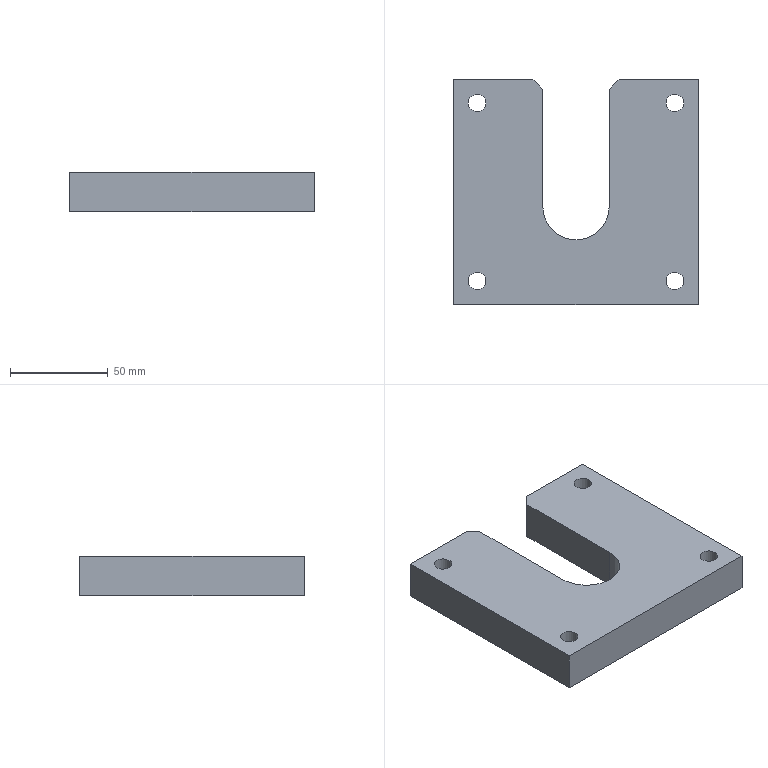Part | NX | features solid 2 | 1 solid | 24 faces | box 125 x 115 x 20 mm | volume 223341 mm3 | plane 15 | cylinder 9 | commonest cylinder face diameters 9.007 x4 14.508 x4 34 x1
STEP:
#1=CARTESIAN_POINT('',(302.977,477.095,246.13));
#2=VERTEX_POINT('',#1);
#3=CARTESIAN_POINT('',(302.977,477.095,226.13));
#4=VERTEX_POINT('',#3);
#5=CARTESIAN_POINT('',(302.977,477.095,221.13));
#6=DIRECTION('',(0.,0.,-1.));
#7=VECTOR('',#6,1000.);
#8=LINE('',#5,#7);
#9=EDGE_CURVE('',#2,#4,#8,.T.);
#10=ORIENTED_EDGE('',*,*,#9,.T.);
#11=CARTESIAN_POINT('',(262.477,477.095,226.13));
#12=VERTEX_POINT('',#11);
#13=CARTESIAN_POINT('',(324.977,477.095,226.13));
#14=DIRECTION('',(1.,0.,0.));
#15=VECTOR('',#14,1000.);
#16=LINE('',#13,#15);
#17=EDGE_CURVE('',#12,#4,#16,.T.);
#18=ORIENTED_EDGE('',*,*,#17,.F.);
#19=CARTESIAN_POINT('',(262.477,477.095,246.13));
#20=VERTEX_POINT('',#19);
#21=CARTESIAN_POINT('',(262.477,477.095,221.13));
#22=DIRECTION('',(0.,0.,1.));
#23=VECTOR('',#22,1000.);
#24=LINE('',#21,#23);
#25=EDGE_CURVE('',#20,#12,#24,.F.);
#26=ORIENTED_EDGE('',*,*,#25,.F.);
#27=CARTESIAN_POINT('',(324.977,477.095,246.13));
#28=DIRECTION('',(1.,0.,0.));
#29=VECTOR('',#28,1000.);
#30=LINE('',#27,#29);
#31=EDGE_CURVE('',#2,#20,#30,.F.);
#32=ORIENTED_EDGE('',*,*,#31,.F.);
#33=EDGE_LOOP('',(#10,#18,#26,#32));
#34=FACE_BOUND('',#33,.T.);
#35=CARTESIAN_POINT('',(324.977,477.095,221.13));
#36=DIRECTION('',(0.,1.,0.));
#37=DIRECTION('',(0.,0.,1.));
#38=AXIS2_PLACEMENT_3D('',#35,#36,#37);
#39=PLANE('',#38);
#40=ADVANCED_FACE('',(#34),#39,.T.);
#41=CARTESIAN_POINT('',(307.977,472.095,226.13));
#42=VERTEX_POINT('',#41);
#43=CARTESIAN_POINT('',(334.227,445.845,226.13));
#44=DIRECTION('',(0.7071,-0.7071,0.));
#45=VECTOR('',#44,1000.);
#46=LINE('',#43,#45);
#47=EDGE_CURVE('',#42,#4,#46,.F.);
#48=ORIENTED_EDGE('',*,*,#47,.F.);
#49=CARTESIAN_POINT('',(307.977,412.095,226.13));
#50=VERTEX_POINT('',#49);
#51=CARTESIAN_POINT('',(307.977,434.595,226.13));
#52=DIRECTION('',(0.,-1.,0.));
#53=VECTOR('',#52,1000.);
#54=LINE('',#51,#53);
#55=EDGE_CURVE('',#42,#50,#54,.T.);
#56=ORIENTED_EDGE('',*,*,#55,.T.);
#57=CARTESIAN_POINT('',(341.977,412.095,226.13));
#58=VERTEX_POINT('',#57);
#59=CARTESIAN_POINT('',(324.977,412.095,226.13));
#60=DIRECTION('',(0.,0.,-1.));
#61=DIRECTION('',(-1.,0.,0.));
#62=AXIS2_PLACEMENT_3D('',#59,#60,#61);
#63=CIRCLE('',#62,17.);
#64=EDGE_CURVE('',#58,#50,#63,.T.);
#65=ORIENTED_EDGE('',*,*,#64,.F.);
#66=CARTESIAN_POINT('',(341.977,472.095,226.13));
#67=VERTEX_POINT('',#66);
#68=CARTESIAN_POINT('',(341.977,434.595,226.13));
#69=DIRECTION('',(0.,1.,0.));
#70=VECTOR('',#69,1000.);
#71=LINE('',#68,#70);
#72=EDGE_CURVE('',#67,#58,#71,.F.);
#73=ORIENTED_EDGE('',*,*,#72,.F.);
#74=CARTESIAN_POINT('',(346.977,477.095,226.13));
#75=VERTEX_POINT('',#74);
#76=CARTESIAN_POINT('',(315.727,445.845,226.13));
#77=DIRECTION('',(0.7071,0.7071,0.));
#78=VECTOR('',#77,1000.);
#79=LINE('',#76,#78);
#80=EDGE_CURVE('',#67,#75,#79,.T.);
#81=ORIENTED_EDGE('',*,*,#80,.T.);
#82=CARTESIAN_POINT('',(387.477,477.095,226.13));
#83=VERTEX_POINT('',#82);
#84=CARTESIAN_POINT('',(324.977,477.095,226.13));
#85=DIRECTION('',(1.,0.,0.));
#86=VECTOR('',#85,1000.);
#87=LINE('',#84,#86);
#88=EDGE_CURVE('',#75,#83,#87,.T.);
#89=ORIENTED_EDGE('',*,*,#88,.T.);
#90=CARTESIAN_POINT('',(387.477,362.095,226.13));
#91=VERTEX_POINT('',#90);
#92=CARTESIAN_POINT('',(387.477,434.595,226.13));
#93=DIRECTION('',(0.,-1.,0.));
#94=VECTOR('',#93,1000.);
#95=LINE('',#92,#94);
#96=EDGE_CURVE('',#83,#91,#95,.T.);
#97=ORIENTED_EDGE('',*,*,#96,.T.);
#98=CARTESIAN_POINT('',(262.477,362.095,226.13));
#99=VERTEX_POINT('',#98);
#100=CARTESIAN_POINT('',(324.977,362.095,226.13));
#101=DIRECTION('',(-1.,0.,0.));
#102=VECTOR('',#101,1000.);
#103=LINE('',#100,#102);
#104=EDGE_CURVE('',#91,#99,#103,.T.);
#105=ORIENTED_EDGE('',*,*,#104,.T.);
#106=CARTESIAN_POINT('',(262.477,434.595,226.13));
#107=DIRECTION('',(0.,1.,0.));
#108=VECTOR('',#107,1000.);
#109=LINE('',#106,#108);
#110=EDGE_CURVE('',#99,#12,#109,.T.);
#111=ORIENTED_EDGE('',*,*,#110,.T.);
#112=ORIENTED_EDGE('',*,*,#17,.T.);
#113=EDGE_LOOP('',(#48,#56,#65,#73,#81,#89,#97,#105,#111,#112));
#114=FACE_BOUND('',#113,.T.);
#115=CARTESIAN_POINT('',(267.223,374.095,226.13));
#116=VERTEX_POINT('',#115);
#117=CARTESIAN_POINT('',(274.477,374.095,226.13));
#118=DIRECTION('',(0.,0.,1.));
#119=DIRECTION('',(-1.,0.,0.));
#120=AXIS2_PLACEMENT_3D('',#117,#118,#119);
#121=CIRCLE('',#120,7.254);
#122=EDGE_CURVE('',#116,#116,#121,.F.);
#123=ORIENTED_EDGE('',*,*,#122,.F.);
#124=EDGE_LOOP('',(#123));
#125=FACE_BOUND('',#124,.T.);
#126=CARTESIAN_POINT('',(267.223,465.095,226.13));
#127=VERTEX_POINT('',#126);
#128=CARTESIAN_POINT('',(274.477,465.095,226.13));
#129=DIRECTION('',(0.,0.,1.));
#130=DIRECTION('',(-1.,0.,0.));
#131=AXIS2_PLACEMENT_3D('',#128,#129,#130);
#132=CIRCLE('',#131,7.254);
#133=EDGE_CURVE('',#127,#127,#132,.F.);
#134=ORIENTED_EDGE('',*,*,#133,.F.);
#135=EDGE_LOOP('',(#134));
#136=FACE_BOUND('',#135,.T.);
#137=CARTESIAN_POINT('',(368.223,374.095,226.13));
#138=VERTEX_POINT('',#137);
#139=CARTESIAN_POINT('',(375.477,374.095,226.13));
#140=DIRECTION('',(0.,0.,1.));
#141=DIRECTION('',(-1.,0.,0.));
#142=AXIS2_PLACEMENT_3D('',#139,#140,#141);
#143=CIRCLE('',#142,7.254);
#144=EDGE_CURVE('',#138,#138,#143,.F.);
#145=ORIENTED_EDGE('',*,*,#144,.F.);
#146=EDGE_LOOP('',(#145));
#147=FACE_BOUND('',#146,.T.);
#148=CARTESIAN_POINT('',(368.223,465.095,226.13));
#149=VERTEX_POINT('',#148);
#150=CARTESIAN_POINT('',(375.477,465.095,226.13));
#151=DIRECTION('',(0.,0.,1.));
#152=DIRECTION('',(-1.,0.,0.));
#153=AXIS2_PLACEMENT_3D('',#150,#151,#152);
#154=CIRCLE('',#153,7.254);
#155=EDGE_CURVE('',#149,#149,#154,.F.);
#156=ORIENTED_EDGE('',*,*,#155,.F.);
#157=EDGE_LOOP('',(#156));
#158=FACE_BOUND('',#157,.T.);
#159=CARTESIAN_POINT('',(324.977,434.595,226.13));
#160=DIRECTION('',(0.,0.,-1.));
#161=DIRECTION('',(0.,1.,0.));
#162=AXIS2_PLACEMENT_3D('',#159,#160,#161);
#163=PLANE('',#162);
#164=ADVANCED_FACE('',(#114,#125,#136,#147,#158),#163,.T.);
#165=CARTESIAN_POINT('',(307.977,472.095,246.13));
#166=VERTEX_POINT('',#165);
#167=CARTESIAN_POINT('',(334.227,445.845,246.13));
#168=DIRECTION('',(-0.7071,0.7071,0.));
#169=VECTOR('',#168,1000.);
#170=LINE('',#167,#169);
#171=EDGE_CURVE('',#2,#166,#170,.F.);
#172=ORIENTED_EDGE('',*,*,#171,.F.);
#173=ORIENTED_EDGE('',*,*,#31,.T.);
#174=CARTESIAN_POINT('',(262.477,362.095,246.13));
#175=VERTEX_POINT('',#174);
#176=CARTESIAN_POINT('',(262.477,434.595,246.13));
#177=DIRECTION('',(0.,1.,0.));
#178=VECTOR('',#177,1000.);
#179=LINE('',#176,#178);
#180=EDGE_CURVE('',#20,#175,#179,.F.);
#181=ORIENTED_EDGE('',*,*,#180,.T.);
#182=CARTESIAN_POINT('',(387.477,362.095,246.13));
#183=VERTEX_POINT('',#182);
#184=CARTESIAN_POINT('',(324.977,362.095,246.13));
#185=DIRECTION('',(1.,0.,0.));
#186=VECTOR('',#185,1000.);
#187=LINE('',#184,#186);
#188=EDGE_CURVE('',#175,#183,#187,.T.);
#189=ORIENTED_EDGE('',*,*,#188,.T.);
#190=CARTESIAN_POINT('',(387.477,477.095,246.13));
#191=VERTEX_POINT('',#190);
#192=CARTESIAN_POINT('',(387.477,434.595,246.13));
#193=DIRECTION('',(0.,-1.,0.));
#194=VECTOR('',#193,1000.);
#195=LINE('',#192,#194);
#196=EDGE_CURVE('',#183,#191,#195,.F.);
#197=ORIENTED_EDGE('',*,*,#196,.T.);
#198=CARTESIAN_POINT('',(346.977,477.095,246.13));
#199=VERTEX_POINT('',#198);
#200=CARTESIAN_POINT('',(324.977,477.095,246.13));
#201=DIRECTION('',(1.,0.,0.));
#202=VECTOR('',#201,1000.);
#203=LINE('',#200,#202);
#204=EDGE_CURVE('',#191,#199,#203,.F.);
#205=ORIENTED_EDGE('',*,*,#204,.T.);
#206=CARTESIAN_POINT('',(341.977,472.095,246.13));
#207=VERTEX_POINT('',#206);
#208=CARTESIAN_POINT('',(315.727,445.845,246.13));
#209=DIRECTION('',(-0.7071,-0.7071,0.));
#210=VECTOR('',#209,1000.);
#211=LINE('',#208,#210);
#212=EDGE_CURVE('',#199,#207,#211,.T.);
#213=ORIENTED_EDGE('',*,*,#212,.T.);
#214=CARTESIAN_POINT('',(341.977,412.095,246.13));
#215=VERTEX_POINT('',#214);
#216=CARTESIAN_POINT('',(341.977,434.595,246.13));
#217=DIRECTION('',(0.,-1.,0.));
#218=VECTOR('',#217,1000.);
#219=LINE('',#216,#218);
#220=EDGE_CURVE('',#207,#215,#219,.T.);
#221=ORIENTED_EDGE('',*,*,#220,.T.);
#222=CARTESIAN_POINT('',(307.977,412.095,246.13));
#223=VERTEX_POINT('',#222);
#224=CARTESIAN_POINT('',(324.977,412.095,246.13));
#225=DIRECTION('',(0.,0.,1.));
#226=DIRECTION('',(1.,0.,0.));
#227=AXIS2_PLACEMENT_3D('',#224,#225,#226);
#228=CIRCLE('',#227,17.);
#229=EDGE_CURVE('',#223,#215,#228,.T.);
#230=ORIENTED_EDGE('',*,*,#229,.F.);
#231=CARTESIAN_POINT('',(307.977,434.595,246.13));
#232=DIRECTION('',(0.,1.,0.));
#233=VECTOR('',#232,1000.);
#234=LINE('',#231,#233);
#235=EDGE_CURVE('',#223,#166,#234,.T.);
#236=ORIENTED_EDGE('',*,*,#235,.T.);
#237=EDGE_LOOP('',(#172,#173,#181,#189,#197,#205,#213,#221,#230,#236));
#238=FACE_BOUND('',#237,.T.);
#239=CARTESIAN_POINT('',(375.477,460.592,246.13));
#240=VERTEX_POINT('',#239);
#241=CARTESIAN_POINT('',(375.477,465.095,246.13));
#242=DIRECTION('',(0.,0.,1.));
#243=DIRECTION('',(0.,-1.,0.));
#244=AXIS2_PLACEMENT_3D('',#241,#242,#243);
#245=CIRCLE('',#244,4.503);
#246=EDGE_CURVE('',#240,#240,#245,.F.);
#247=ORIENTED_EDGE('',*,*,#246,.T.);
#248=EDGE_LOOP('',(#247));
#249=FACE_BOUND('',#248,.T.);
#250=CARTESIAN_POINT('',(274.477,369.592,246.13));
#251=VERTEX_POINT('',#250);
#252=CARTESIAN_POINT('',(274.477,374.095,246.13));
#253=DIRECTION('',(0.,0.,1.));
#254=DIRECTION('',(0.,-1.,0.));
#255=AXIS2_PLACEMENT_3D('',#252,#253,#254);
#256=CIRCLE('',#255,4.503);
#257=EDGE_CURVE('',#251,#251,#256,.F.);
#258=ORIENTED_EDGE('',*,*,#257,.T.);
#259=EDGE_LOOP('',(#258));
#260=FACE_BOUND('',#259,.T.);
#261=CARTESIAN_POINT('',(375.477,369.592,246.13));
#262=VERTEX_POINT('',#261);
#263=CARTESIAN_POINT('',(375.477,374.095,246.13));
#264=DIRECTION('',(0.,0.,1.));
#265=DIRECTION('',(0.,-1.,0.));
#266=AXIS2_PLACEMENT_3D('',#263,#264,#265);
#267=CIRCLE('',#266,4.503);
#268=EDGE_CURVE('',#262,#262,#267,.F.);
#269=ORIENTED_EDGE('',*,*,#268,.T.);
#270=EDGE_LOOP('',(#269));
#271=FACE_BOUND('',#270,.T.);
#272=CARTESIAN_POINT('',(274.477,460.592,246.13));
#273=VERTEX_POINT('',#272);
#274=CARTESIAN_POINT('',(274.477,465.095,246.13));
#275=DIRECTION('',(0.,0.,1.));
#276=DIRECTION('',(0.,-1.,0.));
#277=AXIS2_PLACEMENT_3D('',#274,#275,#276);
#278=CIRCLE('',#277,4.503);
#279=EDGE_CURVE('',#273,#273,#278,.F.);
#280=ORIENTED_EDGE('',*,*,#279,.T.);
#281=EDGE_LOOP('',(#280));
#282=FACE_BOUND('',#281,.T.);
#283=CARTESIAN_POINT('',(324.977,434.595,246.13));
#284=DIRECTION('',(0.,0.,1.));
#285=DIRECTION('',(0.,-1.,0.));
#286=AXIS2_PLACEMENT_3D('',#283,#284,#285);
#287=PLANE('',#286);
#288=ADVANCED_FACE('',(#238,#249,#260,#271,#282),#287,.T.);
#289=CARTESIAN_POINT('',(262.477,362.095,221.13));
#290=DIRECTION('',(0.,0.,-1.));
#291=VECTOR('',#290,1000.);
#292=LINE('',#289,#291);
#293=EDGE_CURVE('',#175,#99,#292,.T.);
#294=ORIENTED_EDGE('',*,*,#293,.F.);
#295=ORIENTED_EDGE('',*,*,#180,.F.);
#296=ORIENTED_EDGE('',*,*,#25,.T.);
#297=ORIENTED_EDGE('',*,*,#110,.F.);
#298=EDGE_LOOP('',(#294,#295,#296,#297));
#299=FACE_BOUND('',#298,.T.);
#300=CARTESIAN_POINT('',(262.477,434.595,221.13));
#301=DIRECTION('',(-1.,0.,0.));
#302=DIRECTION('',(0.,0.,-1.));
#303=AXIS2_PLACEMENT_3D('',#300,#301,#302);
#304=PLANE('',#303);
#305=ADVANCED_FACE('',(#299),#304,.T.);
#306=CARTESIAN_POINT('',(346.977,477.095,221.13));
#307=DIRECTION('',(0.,0.,1.));
#308=VECTOR('',#307,1000.);
#309=LINE('',#306,#308);
#310=EDGE_CURVE('',#75,#199,#309,.T.);
#311=ORIENTED_EDGE('',*,*,#310,.T.);
#312=ORIENTED_EDGE('',*,*,#204,.F.);
#313=CARTESIAN_POINT('',(387.477,477.095,221.13));
#314=DIRECTION('',(0.,0.,1.));
#315=VECTOR('',#314,1000.);
#316=LINE('',#313,#315);
#317=EDGE_CURVE('',#191,#83,#316,.F.);
#318=ORIENTED_EDGE('',*,*,#317,.T.);
#319=ORIENTED_EDGE('',*,*,#88,.F.);
#320=EDGE_LOOP('',(#311,#312,#318,#319));
#321=FACE_BOUND('',#320,.T.);
#322=CARTESIAN_POINT('',(324.977,477.095,221.13));
#323=DIRECTION('',(0.,1.,0.));
#324=DIRECTION('',(0.,0.,1.));
#325=AXIS2_PLACEMENT_3D('',#322,#323,#324);
#326=PLANE('',#325);
#327=ADVANCED_FACE('',(#321),#326,.T.);
#328=ORIENTED_EDGE('',*,*,#317,.F.);
#329=ORIENTED_EDGE('',*,*,#196,.F.);
#330=CARTESIAN_POINT('',(387.477,362.095,221.13));
#331=DIRECTION('',(0.,0.,-1.));
#332=VECTOR('',#331,1000.);
#333=LINE('',#330,#332);
#334=EDGE_CURVE('',#183,#91,#333,.T.);
#335=ORIENTED_EDGE('',*,*,#334,.T.);
#336=ORIENTED_EDGE('',*,*,#96,.F.);
#337=EDGE_LOOP('',(#328,#329,#335,#336));
#338=FACE_BOUND('',#337,.T.);
#339=CARTESIAN_POINT('',(387.477,434.595,221.13));
#340=DIRECTION('',(1.,0.,0.));
#341=DIRECTION('',(0.,0.,1.));
#342=AXIS2_PLACEMENT_3D('',#339,#340,#341);
#343=PLANE('',#342);
#344=ADVANCED_FACE('',(#338),#343,.T.);
#345=ORIENTED_EDGE('',*,*,#104,.F.);
#346=ORIENTED_EDGE('',*,*,#334,.F.);
#347=ORIENTED_EDGE('',*,*,#188,.F.);
#348=ORIENTED_EDGE('',*,*,#293,.T.);
#349=EDGE_LOOP('',(#345,#346,#347,#348));
#350=FACE_BOUND('',#349,.T.);
#351=CARTESIAN_POINT('',(324.977,362.095,221.13));
#352=DIRECTION('',(0.,-1.,0.));
#353=DIRECTION('',(0.,0.,-1.));
#354=AXIS2_PLACEMENT_3D('',#351,#352,#353);
#355=PLANE('',#354);
#356=ADVANCED_FACE('',(#350),#355,.T.);
#357=ORIENTED_EDGE('',*,*,#279,.F.);
#358=EDGE_LOOP('',(#357));
#359=FACE_BOUND('',#358,.T.);
#360=CARTESIAN_POINT('',(274.477,460.592,239.13));
#361=VERTEX_POINT('',#360);
#362=CARTESIAN_POINT('',(274.477,465.095,239.13));
#363=DIRECTION('',(0.,0.,1.));
#364=DIRECTION('',(0.,-1.,0.));
#365=AXIS2_PLACEMENT_3D('',#362,#363,#364);
#366=CIRCLE('',#365,4.503);
#367=EDGE_CURVE('',#361,#361,#366,.F.);
#368=ORIENTED_EDGE('',*,*,#367,.T.);
#369=EDGE_LOOP('',(#368));
#370=FACE_BOUND('',#369,.T.);
#371=CARTESIAN_POINT('',(274.477,465.095,218.13));
#372=DIRECTION('',(0.,0.,1.));
#373=DIRECTION('',(0.,-1.,0.));
#374=AXIS2_PLACEMENT_3D('',#371,#372,#373);
#375=CYLINDRICAL_SURFACE('',#374,4.503);
#376=ADVANCED_FACE('',(#359,#370),#375,.F.);
#377=ORIENTED_EDGE('',*,*,#367,.F.);
#378=EDGE_LOOP('',(#377));
#379=FACE_BOUND('',#378,.T.);
#380=CARTESIAN_POINT('',(274.477,457.841,239.13));
#381=VERTEX_POINT('',#380);
#382=CARTESIAN_POINT('',(274.477,465.095,239.13));
#383=DIRECTION('',(0.,0.,-1.));
#384=DIRECTION('',(0.,-1.,0.));
#385=AXIS2_PLACEMENT_3D('',#382,#383,#384);
#386=CIRCLE('',#385,7.254);
#387=EDGE_CURVE('',#381,#381,#386,.T.);
#388=ORIENTED_EDGE('',*,*,#387,.T.);
#389=EDGE_LOOP('',(#388));
#390=FACE_BOUND('',#389,.T.);
#391=CARTESIAN_POINT('',(274.477,465.095,239.13));
#392=DIRECTION('',(0.,0.,1.));
#393=DIRECTION('',(0.,-1.,0.));
#394=AXIS2_PLACEMENT_3D('',#391,#392,#393);
#395=PLANE('',#394);
#396=ADVANCED_FACE('',(#379,#390),#395,.F.);
#397=ORIENTED_EDGE('',*,*,#387,.F.);
#398=EDGE_LOOP('',(#397));
#399=FACE_BOUND('',#398,.T.);
#400=ORIENTED_EDGE('',*,*,#133,.T.);
#401=EDGE_LOOP('',(#400));
#402=FACE_BOUND('',#401,.T.);
#403=CARTESIAN_POINT('',(274.477,465.095,221.13));
#404=DIRECTION('',(0.,0.,1.));
#405=DIRECTION('',(0.,-1.,0.));
#406=AXIS2_PLACEMENT_3D('',#403,#404,#405);
#407=CYLINDRICAL_SURFACE('',#406,7.254);
#408=ADVANCED_FACE('',(#399,#402),#407,.F.);
#409=ORIENTED_EDGE('',*,*,#268,.F.);
#410=EDGE_LOOP('',(#409));
#411=FACE_BOUND('',#410,.T.);
#412=CARTESIAN_POINT('',(375.477,369.592,239.13));
#413=VERTEX_POINT('',#412);
#414=CARTESIAN_POINT('',(375.477,374.095,239.13));
#415=DIRECTION('',(0.,0.,1.));
#416=DIRECTION('',(0.,-1.,0.));
#417=AXIS2_PLACEMENT_3D('',#414,#415,#416);
#418=CIRCLE('',#417,4.503);
#419=EDGE_CURVE('',#413,#413,#418,.F.);
#420=ORIENTED_EDGE('',*,*,#419,.T.);
#421=EDGE_LOOP('',(#420));
#422=FACE_BOUND('',#421,.T.);
#423=CARTESIAN_POINT('',(375.477,374.095,218.13));
#424=DIRECTION('',(0.,0.,1.));
#425=DIRECTION('',(0.,-1.,0.));
#426=AXIS2_PLACEMENT_3D('',#423,#424,#425);
#427=CYLINDRICAL_SURFACE('',#426,4.503);
#428=ADVANCED_FACE('',(#411,#422),#427,.F.);
#429=ORIENTED_EDGE('',*,*,#419,.F.);
#430=EDGE_LOOP('',(#429));
#431=FACE_BOUND('',#430,.T.);
#432=CARTESIAN_POINT('',(375.477,366.841,239.13));
#433=VERTEX_POINT('',#432);
#434=CARTESIAN_POINT('',(375.477,374.095,239.13));
#435=DIRECTION('',(0.,0.,-1.));
#436=DIRECTION('',(0.,-1.,0.));
#437=AXIS2_PLACEMENT_3D('',#434,#435,#436);
#438=CIRCLE('',#437,7.254);
#439=EDGE_CURVE('',#433,#433,#438,.T.);
#440=ORIENTED_EDGE('',*,*,#439,.T.);
#441=EDGE_LOOP('',(#440));
#442=FACE_BOUND('',#441,.T.);
#443=CARTESIAN_POINT('',(375.477,374.095,239.13));
#444=DIRECTION('',(0.,0.,1.));
#445=DIRECTION('',(0.,-1.,0.));
#446=AXIS2_PLACEMENT_3D('',#443,#444,#445);
#447=PLANE('',#446);
#448=ADVANCED_FACE('',(#431,#442),#447,.F.);
#449=ORIENTED_EDGE('',*,*,#439,.F.);
#450=EDGE_LOOP('',(#449));
#451=FACE_BOUND('',#450,.T.);
#452=ORIENTED_EDGE('',*,*,#144,.T.);
#453=EDGE_LOOP('',(#452));
#454=FACE_BOUND('',#453,.T.);
#455=CARTESIAN_POINT('',(375.477,374.095,221.13));
#456=DIRECTION('',(0.,0.,1.));
#457=DIRECTION('',(0.,-1.,0.));
#458=AXIS2_PLACEMENT_3D('',#455,#456,#457);
#459=CYLINDRICAL_SURFACE('',#458,7.254);
#460=ADVANCED_FACE('',(#451,#454),#459,.F.);
#461=ORIENTED_EDGE('',*,*,#257,.F.);
#462=EDGE_LOOP('',(#461));
#463=FACE_BOUND('',#462,.T.);
#464=CARTESIAN_POINT('',(274.477,369.592,239.13));
#465=VERTEX_POINT('',#464);
#466=CARTESIAN_POINT('',(274.477,374.095,239.13));
#467=DIRECTION('',(0.,0.,1.));
#468=DIRECTION('',(0.,-1.,0.));
#469=AXIS2_PLACEMENT_3D('',#466,#467,#468);
#470=CIRCLE('',#469,4.503);
#471=EDGE_CURVE('',#465,#465,#470,.F.);
#472=ORIENTED_EDGE('',*,*,#471,.T.);
#473=EDGE_LOOP('',(#472));
#474=FACE_BOUND('',#473,.T.);
#475=CARTESIAN_POINT('',(274.477,374.095,218.13));
#476=DIRECTION('',(0.,0.,1.));
#477=DIRECTION('',(0.,-1.,0.));
#478=AXIS2_PLACEMENT_3D('',#475,#476,#477);
#479=CYLINDRICAL_SURFACE('',#478,4.503);
#480=ADVANCED_FACE('',(#463,#474),#479,.F.);
#481=ORIENTED_EDGE('',*,*,#471,.F.);
#482=EDGE_LOOP('',(#481));
#483=FACE_BOUND('',#482,.T.);
#484=CARTESIAN_POINT('',(274.477,366.841,239.13));
#485=VERTEX_POINT('',#484);
#486=CARTESIAN_POINT('',(274.477,374.095,239.13));
#487=DIRECTION('',(0.,0.,-1.));
#488=DIRECTION('',(0.,-1.,0.));
#489=AXIS2_PLACEMENT_3D('',#486,#487,#488);
#490=CIRCLE('',#489,7.254);
#491=EDGE_CURVE('',#485,#485,#490,.T.);
#492=ORIENTED_EDGE('',*,*,#491,.T.);
#493=EDGE_LOOP('',(#492));
#494=FACE_BOUND('',#493,.T.);
#495=CARTESIAN_POINT('',(274.477,374.095,239.13));
#496=DIRECTION('',(0.,0.,1.));
#497=DIRECTION('',(0.,-1.,0.));
#498=AXIS2_PLACEMENT_3D('',#495,#496,#497);
#499=PLANE('',#498);
#500=ADVANCED_FACE('',(#483,#494),#499,.F.);
#501=ORIENTED_EDGE('',*,*,#491,.F.);
#502=EDGE_LOOP('',(#501));
#503=FACE_BOUND('',#502,.T.);
#504=ORIENTED_EDGE('',*,*,#122,.T.);
#505=EDGE_LOOP('',(#504));
#506=FACE_BOUND('',#505,.T.);
#507=CARTESIAN_POINT('',(274.477,374.095,221.13));
#508=DIRECTION('',(0.,0.,1.));
#509=DIRECTION('',(0.,-1.,0.));
#510=AXIS2_PLACEMENT_3D('',#507,#508,#509);
#511=CYLINDRICAL_SURFACE('',#510,7.254);
#512=ADVANCED_FACE('',(#503,#506),#511,.F.);
#513=ORIENTED_EDGE('',*,*,#246,.F.);
#514=EDGE_LOOP('',(#513));
#515=FACE_BOUND('',#514,.T.);
#516=CARTESIAN_POINT('',(375.477,460.592,239.13));
#517=VERTEX_POINT('',#516);
#518=CARTESIAN_POINT('',(375.477,465.095,239.13));
#519=DIRECTION('',(0.,0.,1.));
#520=DIRECTION('',(0.,-1.,0.));
#521=AXIS2_PLACEMENT_3D('',#518,#519,#520);
#522=CIRCLE('',#521,4.503);
#523=EDGE_CURVE('',#517,#517,#522,.F.);
#524=ORIENTED_EDGE('',*,*,#523,.T.);
#525=EDGE_LOOP('',(#524));
#526=FACE_BOUND('',#525,.T.);
#527=CARTESIAN_POINT('',(375.477,465.095,218.13));
#528=DIRECTION('',(0.,0.,1.));
#529=DIRECTION('',(0.,-1.,0.));
#530=AXIS2_PLACEMENT_3D('',#527,#528,#529);
#531=CYLINDRICAL_SURFACE('',#530,4.503);
#532=ADVANCED_FACE('',(#515,#526),#531,.F.);
#533=ORIENTED_EDGE('',*,*,#523,.F.);
#534=EDGE_LOOP('',(#533));
#535=FACE_BOUND('',#534,.T.);
#536=CARTESIAN_POINT('',(375.477,457.841,239.13));
#537=VERTEX_POINT('',#536);
#538=CARTESIAN_POINT('',(375.477,465.095,239.13));
#539=DIRECTION('',(0.,0.,-1.));
#540=DIRECTION('',(0.,-1.,0.));
#541=AXIS2_PLACEMENT_3D('',#538,#539,#540);
#542=CIRCLE('',#541,7.254);
#543=EDGE_CURVE('',#537,#537,#542,.T.);
#544=ORIENTED_EDGE('',*,*,#543,.T.);
#545=EDGE_LOOP('',(#544));
#546=FACE_BOUND('',#545,.T.);
#547=CARTESIAN_POINT('',(375.477,465.095,239.13));
#548=DIRECTION('',(0.,0.,1.));
#549=DIRECTION('',(0.,-1.,0.));
#550=AXIS2_PLACEMENT_3D('',#547,#548,#549);
#551=PLANE('',#550);
#552=ADVANCED_FACE('',(#535,#546),#551,.F.);
#553=ORIENTED_EDGE('',*,*,#543,.F.);
#554=EDGE_LOOP('',(#553));
#555=FACE_BOUND('',#554,.T.);
#556=ORIENTED_EDGE('',*,*,#155,.T.);
#557=EDGE_LOOP('',(#556));
#558=FACE_BOUND('',#557,.T.);
#559=CARTESIAN_POINT('',(375.477,465.095,221.13));
#560=DIRECTION('',(0.,0.,1.));
#561=DIRECTION('',(0.,-1.,0.));
#562=AXIS2_PLACEMENT_3D('',#559,#560,#561);
#563=CYLINDRICAL_SURFACE('',#562,7.254);
#564=ADVANCED_FACE('',(#555,#558),#563,.F.);
#565=ORIENTED_EDGE('',*,*,#47,.T.);
#566=ORIENTED_EDGE('',*,*,#9,.F.);
#567=ORIENTED_EDGE('',*,*,#171,.T.);
#568=CARTESIAN_POINT('',(307.977,472.095,1282.132));
#569=DIRECTION('',(0.,0.,-1.));
#570=VECTOR('',#569,1000.);
#571=LINE('',#568,#570);
#572=EDGE_CURVE('',#42,#166,#571,.F.);
#573=ORIENTED_EDGE('',*,*,#572,.F.);
#574=EDGE_LOOP('',(#565,#566,#567,#573));
#575=FACE_BOUND('',#574,.T.);
#576=CARTESIAN_POINT('',(302.977,477.095,1282.132));
#577=DIRECTION('',(-0.7071,-0.7071,0.));
#578=DIRECTION('',(0.7071,-0.7071,0.));
#579=AXIS2_PLACEMENT_3D('',#576,#577,#578);
#580=PLANE('',#579);
#581=ADVANCED_FACE('',(#575),#580,.F.);
#582=ORIENTED_EDGE('',*,*,#55,.F.);
#583=ORIENTED_EDGE('',*,*,#572,.T.);
#584=ORIENTED_EDGE('',*,*,#235,.F.);
#585=CARTESIAN_POINT('',(307.977,412.095,236.13));
#586=DIRECTION('',(0.,0.,-1.));
#587=VECTOR('',#586,1000.);
#588=LINE('',#585,#587);
#589=EDGE_CURVE('',#50,#223,#588,.F.);
#590=ORIENTED_EDGE('',*,*,#589,.F.);
#591=EDGE_LOOP('',(#582,#583,#584,#590));
#592=FACE_BOUND('',#591,.T.);
#593=CARTESIAN_POINT('',(307.977,472.095,1282.132));
#594=DIRECTION('',(-1.,0.,0.));
#595=DIRECTION('',(0.,0.,1.));
#596=AXIS2_PLACEMENT_3D('',#593,#594,#595);
#597=PLANE('',#596);
#598=ADVANCED_FACE('',(#592),#597,.F.);
#599=ORIENTED_EDGE('',*,*,#64,.T.);
#600=ORIENTED_EDGE('',*,*,#589,.T.);
#601=ORIENTED_EDGE('',*,*,#229,.T.);
#602=CARTESIAN_POINT('',(341.977,412.095,236.13));
#603=DIRECTION('',(0.,0.,-1.));
#604=VECTOR('',#603,1000.);
#605=LINE('',#602,#604);
#606=EDGE_CURVE('',#58,#215,#605,.F.);
#607=ORIENTED_EDGE('',*,*,#606,.F.);
#608=EDGE_LOOP('',(#599,#600,#601,#607));
#609=FACE_BOUND('',#608,.T.);
#610=CARTESIAN_POINT('',(324.977,412.095,1282.132));
#611=DIRECTION('',(0.,0.,-1.));
#612=DIRECTION('',(-1.,0.,0.));
#613=AXIS2_PLACEMENT_3D('',#610,#611,#612);
#614=CYLINDRICAL_SURFACE('',#613,17.);
#615=ADVANCED_FACE('',(#609),#614,.F.);
#616=ORIENTED_EDGE('',*,*,#72,.T.);
#617=ORIENTED_EDGE('',*,*,#606,.T.);
#618=ORIENTED_EDGE('',*,*,#220,.F.);
#619=CARTESIAN_POINT('',(341.977,472.095,1282.132));
#620=DIRECTION('',(0.,0.,-1.));
#621=VECTOR('',#620,1000.);
#622=LINE('',#619,#621);
#623=EDGE_CURVE('',#67,#207,#622,.F.);
#624=ORIENTED_EDGE('',*,*,#623,.F.);
#625=EDGE_LOOP('',(#616,#617,#618,#624));
#626=FACE_BOUND('',#625,.T.);
#627=CARTESIAN_POINT('',(341.977,412.095,1282.132));
#628=DIRECTION('',(1.,0.,0.));
#629=DIRECTION('',(0.,0.,-1.));
#630=AXIS2_PLACEMENT_3D('',#627,#628,#629);
#631=PLANE('',#630);
#632=ADVANCED_FACE('',(#626),#631,.F.);
#633=ORIENTED_EDGE('',*,*,#80,.F.);
#634=ORIENTED_EDGE('',*,*,#623,.T.);
#635=ORIENTED_EDGE('',*,*,#212,.F.);
#636=ORIENTED_EDGE('',*,*,#310,.F.);
#637=EDGE_LOOP('',(#633,#634,#635,#636));
#638=FACE_BOUND('',#637,.T.);
#639=CARTESIAN_POINT('',(341.977,472.095,1282.132));
#640=DIRECTION('',(0.7071,-0.7071,0.));
#641=DIRECTION('',(0.7071,0.7071,0.));
#642=AXIS2_PLACEMENT_3D('',#639,#640,#641);
#643=PLANE('',#642);
#644=ADVANCED_FACE('',(#638),#643,.F.);
#645=CLOSED_SHELL('',(#40,#164,#288,#305,#327,#344,#356,#376,#396,#408,#428,#448,#460,#480,#500,#512,#532,#552,#564,#581,#598,#615,#632,#644));
#646=MANIFOLD_SOLID_BREP('',#645);
#647=(LENGTH_UNIT()NAMED_UNIT(*)SI_UNIT(.MILLI.,.METRE.));
#648=UNCERTAINTY_MEASURE_WITH_UNIT(LENGTH_MEASURE(0.00001),#647,'','');
#649=(NAMED_UNIT(*)PLANE_ANGLE_UNIT()SI_UNIT($,.RADIAN.));
#650=(NAMED_UNIT(*)SI_UNIT($,.STERADIAN.)SOLID_ANGLE_UNIT());
#651=(GEOMETRIC_REPRESENTATION_CONTEXT(3)GLOBAL_UNCERTAINTY_ASSIGNED_CONTEXT((#648))GLOBAL_UNIT_ASSIGNED_CONTEXT((#647,#649,#650))REPRESENTATION_CONTEXT('',''));
#652=ADVANCED_BREP_SHAPE_REPRESENTATION('',(#646),#651);